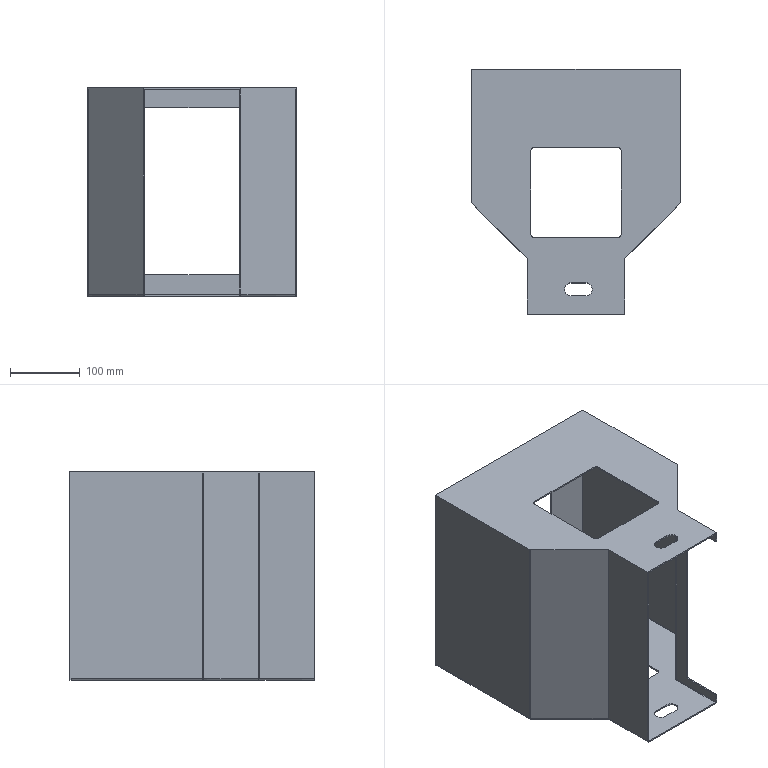Part | STEP file | MYT-A01-P19 | 1 solid | 86 faces | box 300 x 352 x 300 mm | volume 782143 mm3 | plane 52 | cylinder 26 | spline 8 | commonest cylinder face diameters 10 x8 1.473 x6 5.473 x6 18.922 x6